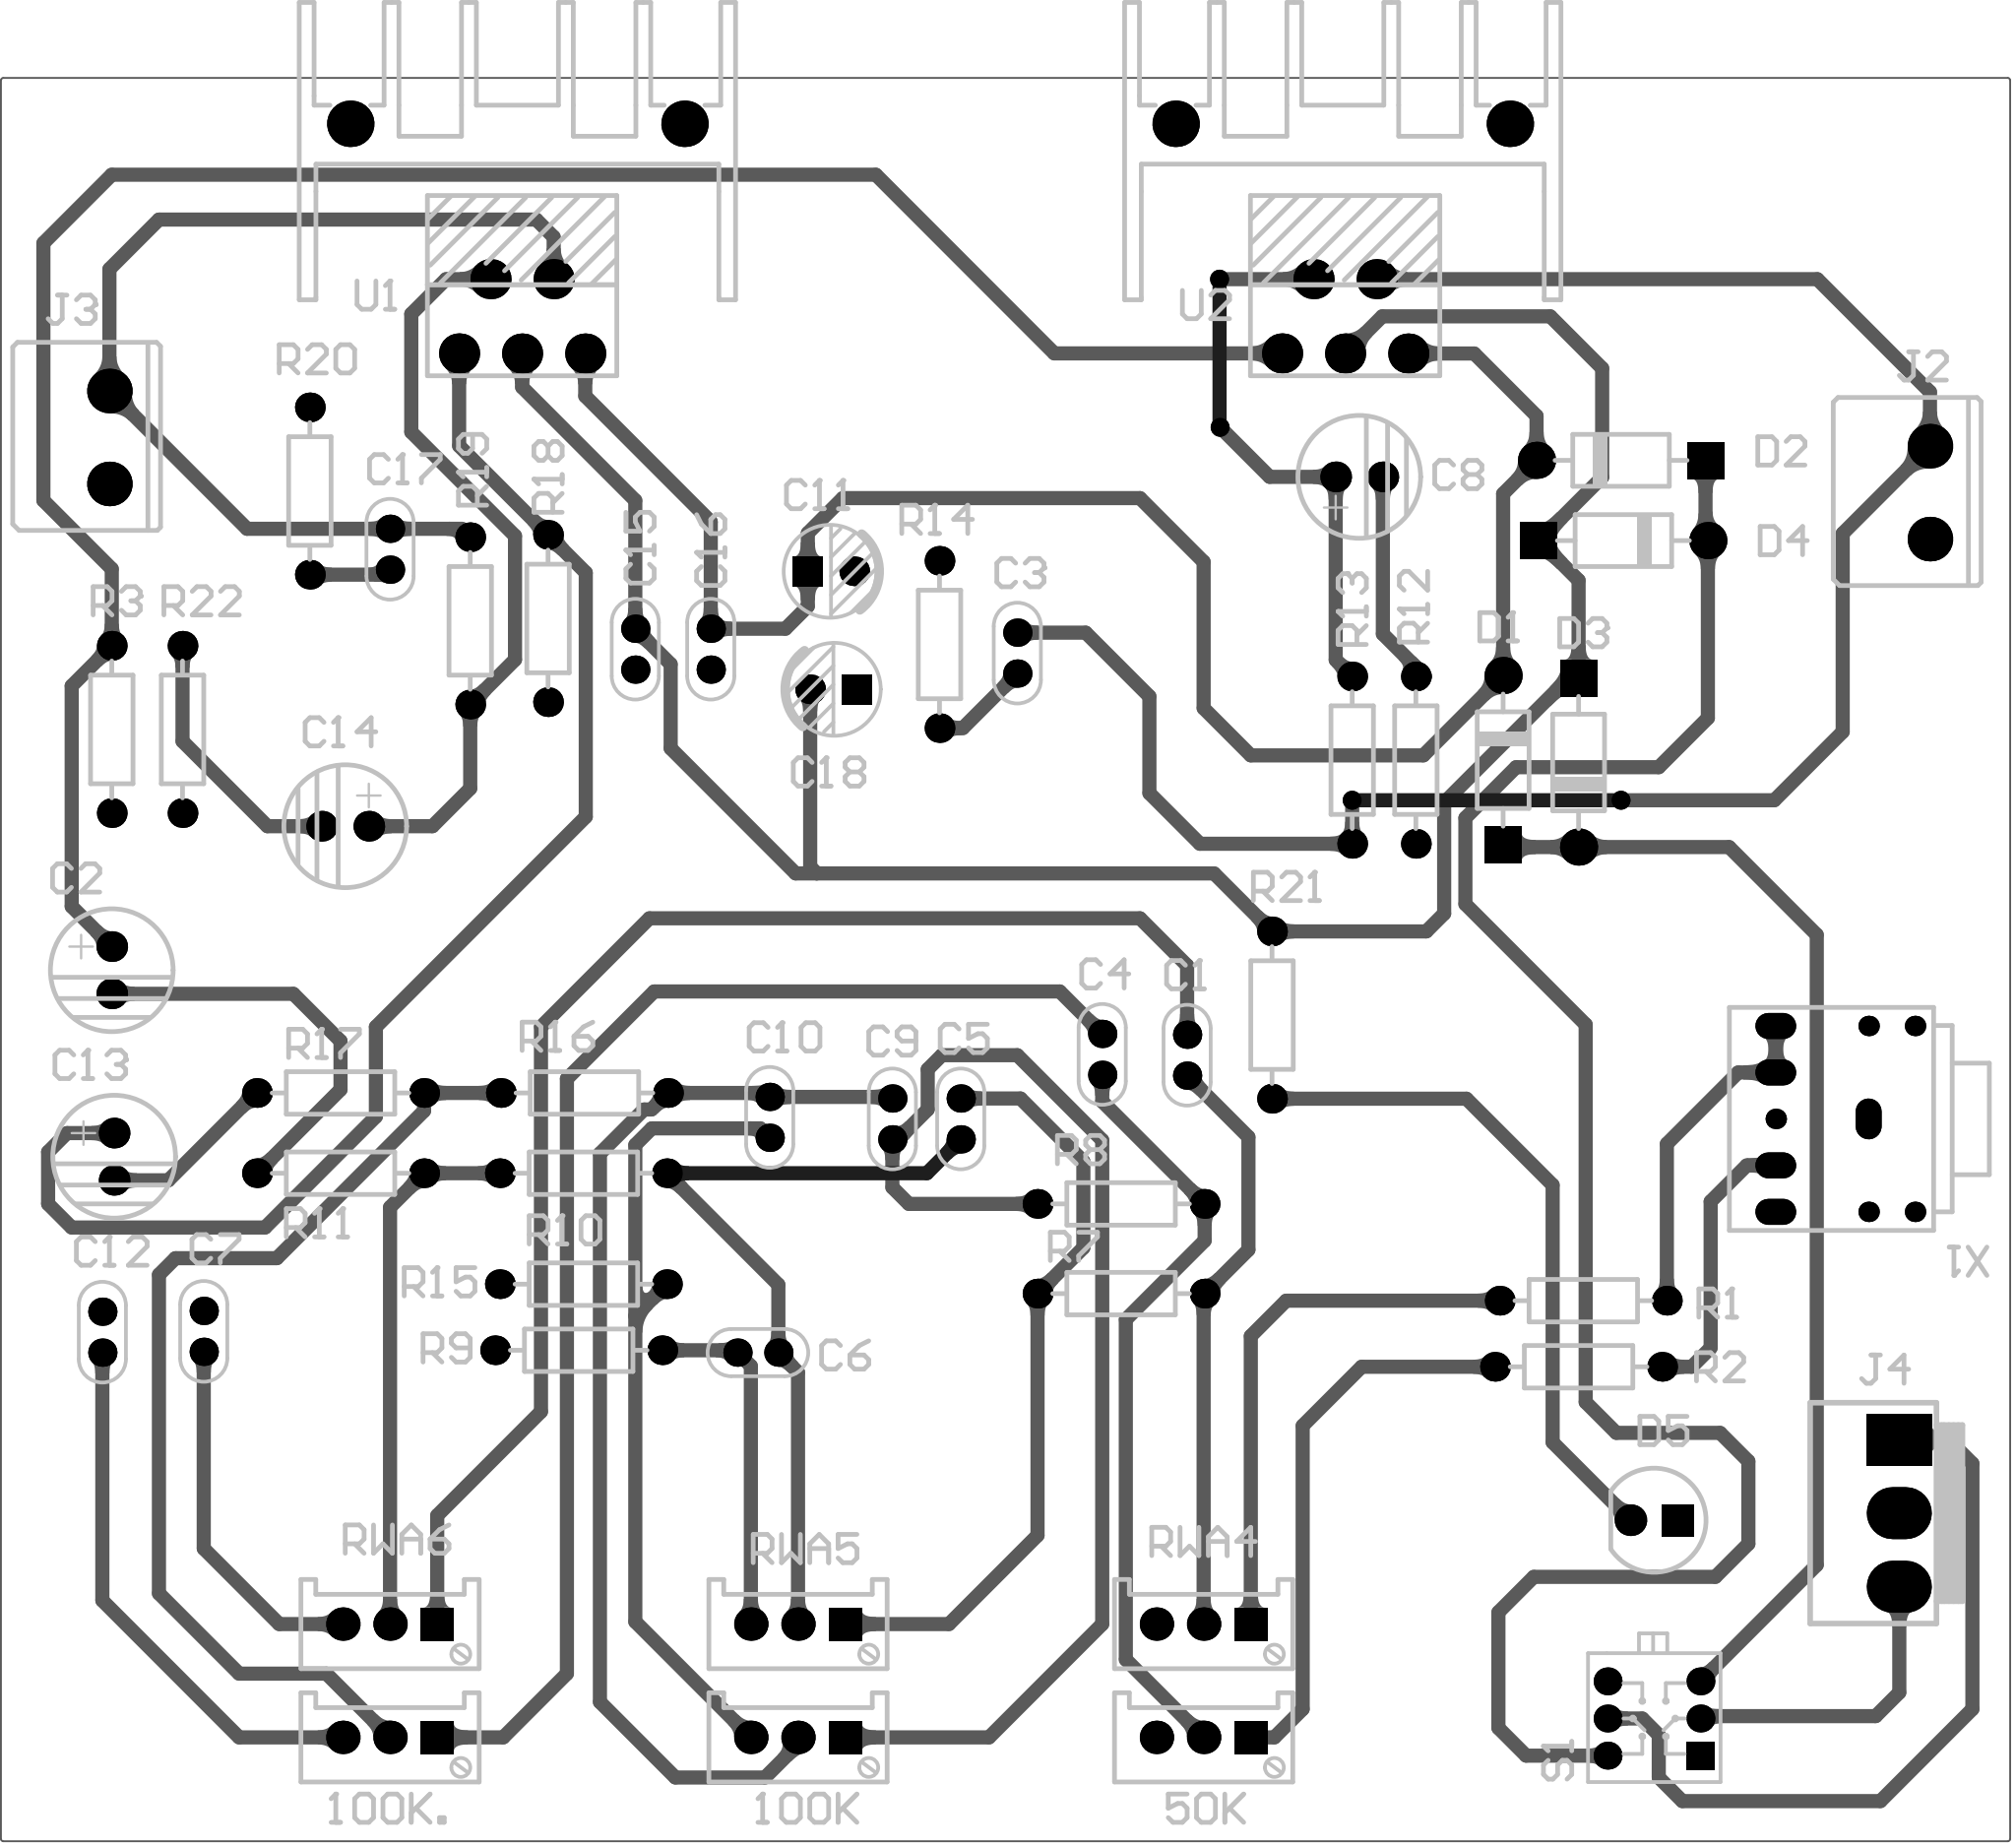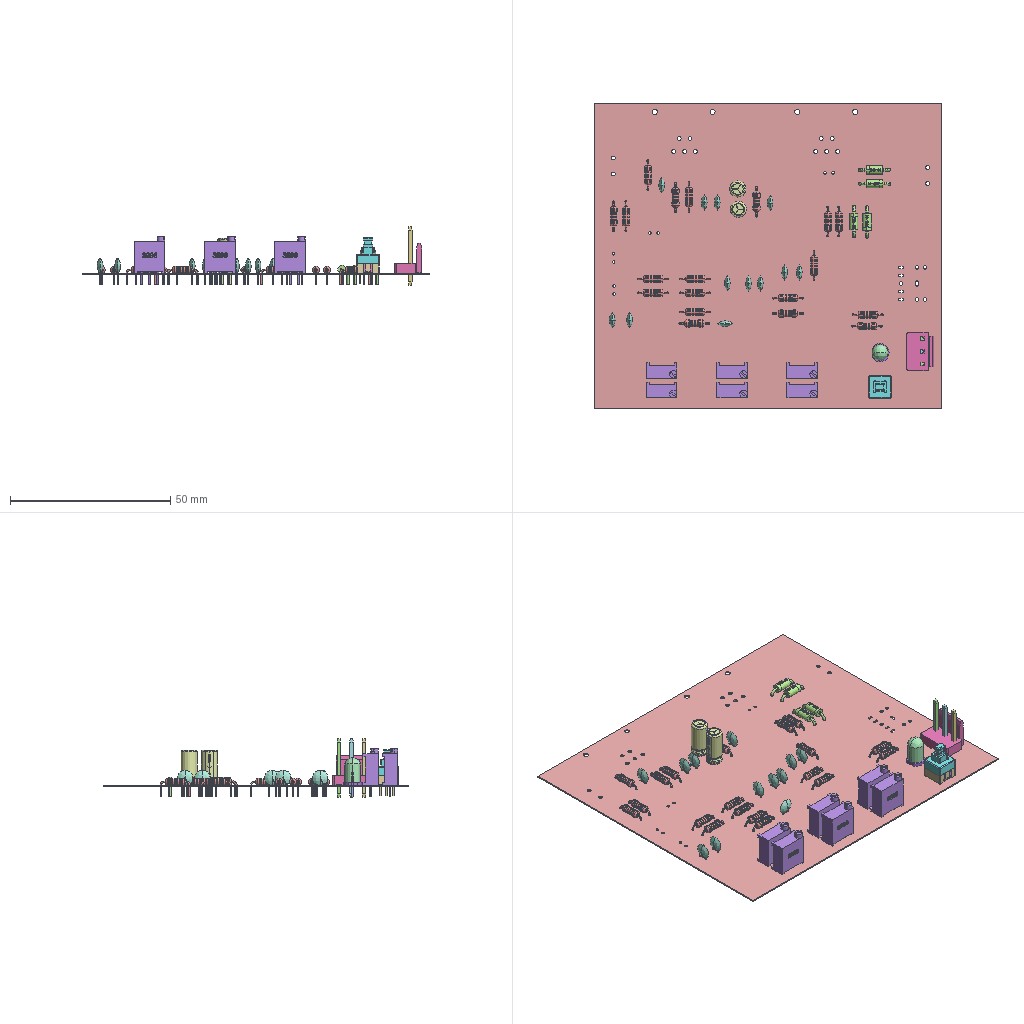Circuit board layout | Altium Designer | box 108.2 x 94.9 x 18.2 mm
Layer stack:
# Altium Designer layer stack of  (unit mm; dielectric type: 0 none, 1 core, 2 prepreg, 3 surface material)
index,name,kind,layer,copper_thickness_mm,dielectric_type,dielectric_thickness_mm,dielectric_material,dielectric_constant
0,Top Paste,other,,,,,,
1,Top Overlay,other,,,,,,
2,Top Solder,dielectric,,,3,0.0102,Solder Resist,3.5
3,Top Layer,copper,Top Layer,0.0356,,,,
4,Dielectric 1,dielectric,,,0,0.32,FR-4,4.8
5,Bottom Layer,copper,Bottom Layer,0.0356,,,,
6,Bottom Solder,dielectric,,,3,0.0102,Solder Resist,3.5
7,Bottom Overlay,other,,,,,,
8,Bottom Paste,other,,,,,,
# drill layer pairs: low layer,high layer
drill_pair,Top Layer,Bottom Layer
Part placement:
Designator,Comment,Layer,Footprint,Center-X(mm),Center-Y(mm),Rotation
X1,STEREO,TopLayer,3F07,124.607,71.755,180
U2,TDA2030,TopLayer,TDA2030,97.667,114.936,0
U1,TDA2030,TopLayer,TDA2030,53.344,114.936,0
S1,KET 7X7,TopLayer,KFT_DIP-7X7,114.3,39.497,90
RWA6,10K,TopLayer,3296W,46.228,44.577,180
RWA5,10K,TopLayer,3296W,68.199,44.577,180
RWA4,10K,TopLayer,3296W,90.043,44.577,180
R22,330,TopLayer,RS_1/4W,35.052,92.71,90
R21,10K,TopLayer,RS_1/4W,93.726,77.343,90
R20,10,TopLayer,RS_1/4W,41.91,105.537,270
R19,47K,TopLayer,RS_1/4W,50.546,98.552,270
R18,22K,TopLayer,RS_1/4W,54.737,98.679,90
R17,2.2K,TopLayer,RS_1/4W,43.561,73.152,180
R16,5.6K,TopLayer,RS_1/4W,56.697,73.152,180
R15,1.5K,TopLayer,RS_1/4W,56.642,62.865,180
R14,10,TopLayer,RS_1/4W,75.819,97.282,270
R13,47K,TopLayer,RS_1/4W,98.044,91.059,90
R12,330,TopLayer,RS_1/4W,101.473,91.059,90
R11,2.2K,TopLayer,RS_1/4W,43.561,68.834,180
R10,5.6K,TopLayer,RS_1/4W,56.642,68.834,180
R9,1.5K,TopLayer,RS_1/4W,56.388,59.309,180
R8,10K,TopLayer,RS_1/4W,85.598,67.183,180
R7,10K,TopLayer,RS_1/4W,85.598,62.357,180
R3,22K,TopLayer,RS_1/4W,31.242,92.71,90
R2,1K,TopLayer,RS_1/4W,110.236,58.42,360
R1,1K,TopLayer,RS_1/4W,110.49,61.976,360
J4,AC+/-12V,TopLayer,VH3.96-3A,127.508,50.546,270
J3,socket,TopLayer,DZ,31.115,108.418,90
J2,socket,TopLayer,DZ,129.159,105.45,90
D5,LED,TopLayer,LED_5MM-W,114.3,50.165,180
D4,1N4007,TopLayer,DO-41,112.649,102.87,360
D3,1N4007,TopLayer,DO-41,110.236,90.932,270
D2,1N4007,TopLayer,DO-41,112.522,107.188,180
D1,1N4007,TopLayer,DO-41,106.172,91.059,90
C18,2200UF,TopLayer,CAP_2.5*5*11_-_BK,70.104,94.869,180
C17,224,TopLayer,CC_2.2*5,46.228,102.405,90
C16,104,TopLayer,CC_2.2*5,63.5,97.028,90
C15,104,TopLayer,CC_2.2*5,59.436,97.028,90
C14,10UF,TopLayer,EC100,43.815,87.503,270
C13,10UF,TopLayer,EC100,31.369,69.723,0
C12,223,TopLayer,CC_2.2*5,30.734,60.282,270
C11,2200UF,TopLayer,CAP_2.5*5*11_-_BK,69.977,101.219,0
C10,224,TopLayer,CC_2.2*5,66.675,71.839,90
C9,223,TopLayer,CC_2.2*5,73.279,71.755,270
C8,10UF,TopLayer,EC100,98.425,106.299,90
C7,223,TopLayer,CC_2.2*5,36.195,60.325,270
C6,224,TopLayer,CC_2.2*5,66.04,59.182,360
C5,223,TopLayer,CC_2.2*5,76.962,71.755,90
C4,222,TopLayer,CC_2.2*5,84.582,75.227,90
C3,224,TopLayer,CC_2.2*5,80.01,96.817,90
C2,10UF,TopLayer,EC100,31.242,79.756,0
C1,222,TopLayer,CC_2.2*5,89.154,75.184,90
100K,10K,TopLayer,3296W,68.199,38.481,180
100K.,10K,TopLayer,3296W,46.228,38.481,180
50K,10K,TopLayer,3296W,90.043,38.481,180
Designator30,Comment,TopLayer,TH-2P_L23.5-W16.8,97.537,125.295,360
Designator31,Comment,TopLayer,TH-2P_L23.5-W16.8,53.087,125.295,360
Pad and via stacks:
# Altium Designer via and pad stacks of  (unit mm). Each distinct definition once, with the count of objects using it.
# via: kind,start_layer,end_layer,hole_mm,diameter_mm,mode(0 simple;1 top-mid-bottom;2 full stack),diameter_per_layer,count,example_net
# pad: kind,layer,hole_mm,hole_type(0 round;1 square;2 slot),plating,top_size,top_shape(1 round;2 rect;3 octagon;9 rounded rect),mid_size,bottom_size,mode,footprint,size_per_layer,count,example
pad,Multi-Layer,1.1,0,unplated,1.1x1.1,1,1.1x1.1,1.1x1.1,0,3F07,,5,X1.
pad,Multi-Layer,0.8,2,plated,2.2x1.4,1,2.2x1.4,2.2x1.4,0,3F07,,5,X1.1
pad,Multi-Layer,0.6,0,plated,1.6x1.6,1,1.6x1.6,1.6x1.6,0,RS 1/4W,,38,R1.2
pad,Multi-Layer,1.2,0,plated,2.4x2.4,1,2.4x2.4,2.4x2.4,0,DZ,,4,J2.1
pad,Multi-Layer,1.2,0,plated,2.159x2.159,1,2.159x2.159,2.159x2.159,0,TDA2030,,10,U2.5
pad,Multi-Layer,0.8128,0,plated,1.651x1.651,1,1.651x1.651,1.651x1.651,0,EC100,,8,C2.1
pad,Multi-Layer,0.5,0,plated,1.524x1.524,1,1.524x1.524,1.524x1.524,0,CC 2.2*5,,24,C3.2
pad,Multi-Layer,0.7,0,plated,1.8x1.8,1,1.8x1.8,1.8x1.8,0,3296W,,12,RWA4.3
pad,Multi-Layer,0.7,0,plated,1.8x1.8,2,1.8x1.8,1.8x1.8,0,3296W,,6,RWA4.1
pad,Multi-Layer,0.8,0,plated,1.6x1.6,1,1.6x1.6,1.6x1.6,0,CAP 2.5*5*11 - BK,,2,C11.2
pad,Multi-Layer,0.8,0,plated,1.6x1.6,2,1.6x1.6,1.6x1.6,0,CAP 2.5*5*11 - BK,,2,C11.1
pad,Multi-Layer,1,0,plated,2x2,1,2x2,2x2,0,DO-41,,4,D2.2
pad,Multi-Layer,1,0,plated,2x2,2,2x2,2x2,0,DO-41,,4,D2.1
pad,Multi-Layer,0.9,0,plated,1.5x1.5,1,1.5x1.5,1.5x1.5,0,KFT DIP-7X7,,5,S1.4
pad,Multi-Layer,0.9,0,plated,1.5x1.5,2,1.5x1.5,1.5x1.5,0,KFT DIP-7X7,,1,S1.1
pad,Multi-Layer,1.6,0,plated,2.8x3.5,1,2.8x3.5,2.8x3.5,0,VH3.96-3A,,2,J4.3
pad,Multi-Layer,1.6,0,plated,2.8x3.5,2,2.8x3.5,2.8x3.5,0,VH3.96-3A,,1,J4.1
pad,Multi-Layer,0.9,0,plated,1.7x1.7,1,1.7x1.7,1.7x1.7,0,LED 5MM-W,,1,D5.2
pad,Multi-Layer,0.9,0,plated,1.7x1.7,2,1.7x1.7,1.7x1.7,0,LED 5MM-W,,1,D5.1
pad,Multi-Layer,1.6,0,plated,2.5x2.5,1,2.5x2.5,2.5x2.5,0,TH-2P_L23.5-W16.8,,4,Designator30.1
via,Top Layer,Bottom Layer,0.508,1.016,0,,4,NetC8_1
Design rules, without the lines most boards share:
# Altium Designer design rules of  (exported by Altium Designer, unit mm)
# columns: name | kind | enabled | priority | scope1 | scope2 | descriptor | typed fields (field=value)
SilkToSilkClearance | 55 | enabled | 1 | All | All | Silk to Silk (Clearance=0mil) (All),(All) |
SilkToSolderMaskClearance | 54 | enabled | 1 | IsPad | All | Silk To Solder Mask (Clearance=9mil) (IsPad),(All) |
MinimumSolderMaskSliver | 53 | enabled | 1 | All | All | Minimum Solder Mask Sliver (Gap=9mil) (All),(All) |
HoleToHoleClearance | 52 | enabled | 1 | All | All | Hole To Hole Clearance (Gap=10mil) (All),(All) | gap=0.254
DiffPairsRouting | 51 | enabled | 1 | All | All | Differential Pairs Uncoupled Length using the Gap Constraints (Min=10mil) (Max=10mil) (Prefered=10mil)  and Width Constraints (Min=15mil) (Max=15mil) (Prefered=15mil) (All) |
HoleSize | 42 | enabled | 1 | All | All | Hole Size Constraint (Min=1mil) (Max=9999mil) (All) |
SolderMaskExpansion | 13 | enabled | 1 | All | All | Solder Mask Expansion (Expansion =4mil) (All) | expansion=0.1016
PasteMaskExpansion | 14 | enabled | 1 | All | All | Paste Mask Expansion (Expansion =0mil) (All) | expansion=0
RoutingVias | 11 | enabled | 1 | All | All | Routing Via (MinHoleWidth=28mil) (MaxHoleWidth=28mil) (PreferredHoleWidth=28mil) (MinWidth=50mil) (MaxWidth=50mil) (PreferedWidth=50mil) (All) | via_min_hole=0.7112 via_max_hole=0.7112 via_preferred_diameter=1.27 via_preferred_hole=0.7112
Width | 2 | enabled | 1 | All | All | Width Constraint (Min=10mil) (Max=30mil) (Preferred=10mil) (All) |
PolygonConnect | 20 | enabled | 1 | All | All | Polygon Connect Rule(Relief Connect )(Conductor Width=10mil) (Relief Angle=90 Angle) (Entries=4) (Air Gap Width=10mil) (All),(All) | connect_style(0=relief,1=direct,2=none)=0 relief_conductor_width=0.254 relief_entries=4
PlaneConnect | 6 | enabled | 1 | All | All | Power Plane Connect Rule(Relief Connect )(Expansion=20mil) (Conductor Width=10mil) (Air Gap=10mil) (Entries=4) (All) | relief_conductor_width=0.254 relief_entries=4 relief_expansion=0.508
Clearance | 0 | enabled | 1 | All | All | Clearance Constraint (Gap=10mil) (All),(All) | gap=0.254
Classes set for this board:
# Altium Designer classes of  (member kind: 0 net, 1 component, 2 from-to, 3 pad, 4 layer, 5 differential pair, 6 design channel, 7 polygon, 8 structure, 9 xSignal)
# columns: class name | member kind | superclass | members
Sheet1 | 1 | no | 50K; 100K; 100K.; C1; C2; C3; C4; C5; C6; C7; C8; C9; C10; C11; C12; C13; C14; C15; C16; C17; C18; D1; D2; D3; D4; D5; J2; J3; J4; R1; R2; R3; R7; R8; R9; R10; R11; R12; R13; R14; R15; R16; R17; R18; R19; R20; R21; R22; RWA4; RWA5; RWA6; S1; U1; U2; X1;